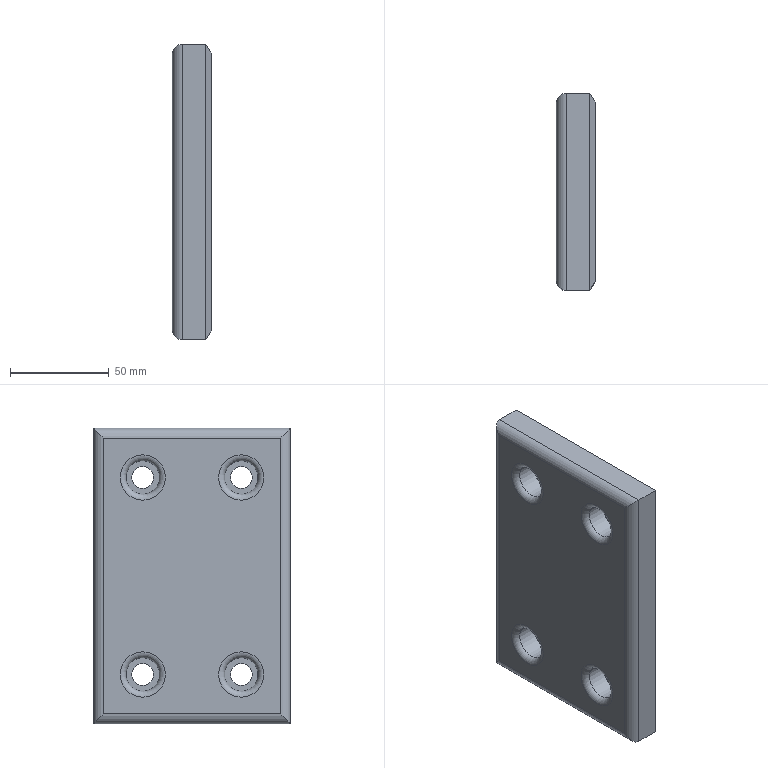Part | NX | features solid 2 | 1 solid | 30 faces | box 20 x 100 x 150 mm | volume 278806 mm3 | plane 14 | cylinder 12 | torus 4 | commonest cylinder face diameters 10 x4 11 x4 17 x4
STEP:
#1=CARTESIAN_POINT('',(-1412.,120.,-125.5));
#2=VERTEX_POINT('',#1);
#3=CARTESIAN_POINT('',(-1412.,120.,-120.));
#4=DIRECTION('',(1.,0.,0.));
#5=DIRECTION('',(0.,0.,-1.));
#6=AXIS2_PLACEMENT_3D('',#3,#4,#5);
#7=CIRCLE('',#6,5.5);
#8=EDGE_CURVE('',#2,#2,#7,.T.);
#9=ORIENTED_EDGE('',*,*,#8,.T.);
#10=EDGE_LOOP('',(#9));
#11=FACE_BOUND('',#10,.T.);
#12=CARTESIAN_POINT('',(-1412.,120.,-128.5));
#13=VERTEX_POINT('',#12);
#14=CARTESIAN_POINT('',(-1412.,120.,-120.));
#15=DIRECTION('',(1.,0.,0.));
#16=DIRECTION('',(0.,0.,-1.));
#17=AXIS2_PLACEMENT_3D('',#14,#15,#16);
#18=CIRCLE('',#17,8.5);
#19=EDGE_CURVE('',#13,#13,#18,.T.);
#20=ORIENTED_EDGE('',*,*,#19,.F.);
#21=EDGE_LOOP('',(#20));
#22=FACE_BOUND('',#21,.T.);
#23=CARTESIAN_POINT('',(-1412.,120.,-120.));
#24=DIRECTION('',(1.,0.,0.));
#25=DIRECTION('',(0.,0.,-1.));
#26=AXIS2_PLACEMENT_3D('',#23,#24,#25);
#27=PLANE('',#26);
#28=ADVANCED_FACE('',(#11,#22),#27,.F.);
#29=CARTESIAN_POINT('',(-1412.,70.,-125.5));
#30=VERTEX_POINT('',#29);
#31=CARTESIAN_POINT('',(-1412.,70.,-120.));
#32=DIRECTION('',(1.,0.,0.));
#33=DIRECTION('',(0.,0.,-1.));
#34=AXIS2_PLACEMENT_3D('',#31,#32,#33);
#35=CIRCLE('',#34,5.5);
#36=EDGE_CURVE('',#30,#30,#35,.T.);
#37=ORIENTED_EDGE('',*,*,#36,.T.);
#38=EDGE_LOOP('',(#37));
#39=FACE_BOUND('',#38,.T.);
#40=CARTESIAN_POINT('',(-1412.,70.,-128.5));
#41=VERTEX_POINT('',#40);
#42=CARTESIAN_POINT('',(-1412.,70.,-120.));
#43=DIRECTION('',(1.,0.,0.));
#44=DIRECTION('',(0.,0.,-1.));
#45=AXIS2_PLACEMENT_3D('',#42,#43,#44);
#46=CIRCLE('',#45,8.5);
#47=EDGE_CURVE('',#41,#41,#46,.T.);
#48=ORIENTED_EDGE('',*,*,#47,.F.);
#49=EDGE_LOOP('',(#48));
#50=FACE_BOUND('',#49,.T.);
#51=CARTESIAN_POINT('',(-1412.,70.,-120.));
#52=DIRECTION('',(1.,0.,0.));
#53=DIRECTION('',(0.,0.,-1.));
#54=AXIS2_PLACEMENT_3D('',#51,#52,#53);
#55=PLANE('',#54);
#56=ADVANCED_FACE('',(#39,#50),#55,.F.);
#57=CARTESIAN_POINT('',(-1422.,120.,-111.5));
#58=VERTEX_POINT('',#57);
#59=CARTESIAN_POINT('',(-1422.,120.,-120.));
#60=DIRECTION('',(-1.,0.,0.));
#61=DIRECTION('',(0.,0.,1.));
#62=AXIS2_PLACEMENT_3D('',#59,#60,#61);
#63=CIRCLE('',#62,8.5);
#64=EDGE_CURVE('',#58,#58,#63,.T.);
#65=ORIENTED_EDGE('',*,*,#64,.T.);
#66=EDGE_LOOP('',(#65));
#67=FACE_BOUND('',#66,.T.);
#68=ORIENTED_EDGE('',*,*,#19,.T.);
#69=EDGE_LOOP('',(#68));
#70=FACE_BOUND('',#69,.T.);
#71=CARTESIAN_POINT('',(-1425.,120.,-120.));
#72=DIRECTION('',(1.,0.,0.));
#73=DIRECTION('',(0.,0.,-1.));
#74=AXIS2_PLACEMENT_3D('',#71,#72,#73);
#75=CYLINDRICAL_SURFACE('',#74,8.5);
#76=ADVANCED_FACE('',(#67,#70),#75,.F.);
#77=CARTESIAN_POINT('',(-1422.,70.,-111.5));
#78=VERTEX_POINT('',#77);
#79=CARTESIAN_POINT('',(-1422.,70.,-120.));
#80=DIRECTION('',(-1.,0.,0.));
#81=DIRECTION('',(0.,0.,1.));
#82=AXIS2_PLACEMENT_3D('',#79,#80,#81);
#83=CIRCLE('',#82,8.5);
#84=EDGE_CURVE('',#78,#78,#83,.T.);
#85=ORIENTED_EDGE('',*,*,#84,.T.);
#86=EDGE_LOOP('',(#85));
#87=FACE_BOUND('',#86,.T.);
#88=ORIENTED_EDGE('',*,*,#47,.T.);
#89=EDGE_LOOP('',(#88));
#90=FACE_BOUND('',#89,.T.);
#91=CARTESIAN_POINT('',(-1425.,70.,-120.));
#92=DIRECTION('',(1.,0.,0.));
#93=DIRECTION('',(0.,0.,-1.));
#94=AXIS2_PLACEMENT_3D('',#91,#92,#93);
#95=CYLINDRICAL_SURFACE('',#94,8.5);
#96=ADVANCED_FACE('',(#87,#90),#95,.F.);
#97=ORIENTED_EDGE('',*,*,#8,.F.);
#98=EDGE_LOOP('',(#97));
#99=FACE_BOUND('',#98,.T.);
#100=CARTESIAN_POINT('',(-1405.,120.,-114.5));
#101=VERTEX_POINT('',#100);
#102=CARTESIAN_POINT('',(-1405.,120.,-120.));
#103=DIRECTION('',(-1.,0.,0.));
#104=DIRECTION('',(0.,0.,1.));
#105=AXIS2_PLACEMENT_3D('',#102,#103,#104);
#106=CIRCLE('',#105,5.5);
#107=EDGE_CURVE('',#101,#101,#106,.T.);
#108=ORIENTED_EDGE('',*,*,#107,.F.);
#109=EDGE_LOOP('',(#108));
#110=FACE_BOUND('',#109,.T.);
#111=CARTESIAN_POINT('',(-1375.,120.,-120.));
#112=DIRECTION('',(1.,0.,0.));
#113=DIRECTION('',(0.,0.,-1.));
#114=AXIS2_PLACEMENT_3D('',#111,#112,#113);
#115=CYLINDRICAL_SURFACE('',#114,5.5);
#116=ADVANCED_FACE('',(#99,#110),#115,.F.);
#117=ORIENTED_EDGE('',*,*,#36,.F.);
#118=EDGE_LOOP('',(#117));
#119=FACE_BOUND('',#118,.T.);
#120=CARTESIAN_POINT('',(-1405.,70.,-114.5));
#121=VERTEX_POINT('',#120);
#122=CARTESIAN_POINT('',(-1405.,70.,-120.));
#123=DIRECTION('',(-1.,0.,0.));
#124=DIRECTION('',(0.,0.,1.));
#125=AXIS2_PLACEMENT_3D('',#122,#123,#124);
#126=CIRCLE('',#125,5.5);
#127=EDGE_CURVE('',#121,#121,#126,.T.);
#128=ORIENTED_EDGE('',*,*,#127,.F.);
#129=EDGE_LOOP('',(#128));
#130=FACE_BOUND('',#129,.T.);
#131=CARTESIAN_POINT('',(-1375.,70.,-120.));
#132=DIRECTION('',(1.,0.,0.));
#133=DIRECTION('',(0.,0.,-1.));
#134=AXIS2_PLACEMENT_3D('',#131,#132,#133);
#135=CYLINDRICAL_SURFACE('',#134,5.5);
#136=ADVANCED_FACE('',(#119,#130),#135,.F.);
#137=CARTESIAN_POINT('',(-1420.,145.,-145.));
#138=VERTEX_POINT('',#137);
#139=CARTESIAN_POINT('',(-1408.,145.,-145.));
#140=VERTEX_POINT('',#139);
#141=CARTESIAN_POINT('',(-1425.,145.,-145.));
#142=DIRECTION('',(-1.,0.,0.));
#143=VECTOR('',#142,1000.);
#144=LINE('',#141,#143);
#145=EDGE_CURVE('',#138,#140,#144,.F.);
#146=ORIENTED_EDGE('',*,*,#145,.T.);
#147=CARTESIAN_POINT('',(-1408.,45.,-145.));
#148=VERTEX_POINT('',#147);
#149=CARTESIAN_POINT('',(-1408.,135.,-145.));
#150=DIRECTION('',(0.,1.,0.));
#151=VECTOR('',#150,1000.);
#152=LINE('',#149,#151);
#153=EDGE_CURVE('',#140,#148,#152,.F.);
#154=ORIENTED_EDGE('',*,*,#153,.T.);
#155=CARTESIAN_POINT('',(-1420.,45.,-145.));
#156=VERTEX_POINT('',#155);
#157=CARTESIAN_POINT('',(-1425.,45.,-145.));
#158=DIRECTION('',(-1.,0.,0.));
#159=VECTOR('',#158,1000.);
#160=LINE('',#157,#159);
#161=EDGE_CURVE('',#156,#148,#160,.F.);
#162=ORIENTED_EDGE('',*,*,#161,.F.);
#163=CARTESIAN_POINT('',(-1420.,145.,-145.));
#164=DIRECTION('',(0.,1.,0.));
#165=VECTOR('',#164,1000.);
#166=LINE('',#163,#165);
#167=EDGE_CURVE('',#156,#138,#166,.T.);
#168=ORIENTED_EDGE('',*,*,#167,.T.);
#169=EDGE_LOOP('',(#146,#154,#162,#168));
#170=FACE_BOUND('',#169,.T.);
#171=CARTESIAN_POINT('',(-1415.,135.,-145.));
#172=DIRECTION('',(0.,0.,-1.));
#173=DIRECTION('',(0.,-1.,0.));
#174=AXIS2_PLACEMENT_3D('',#171,#172,#173);
#175=PLANE('',#174);
#176=ADVANCED_FACE('',(#170),#175,.T.);
#177=ORIENTED_EDGE('',*,*,#64,.F.);
#178=EDGE_LOOP('',(#177));
#179=FACE_BOUND('',#178,.T.);
#180=CARTESIAN_POINT('',(-1425.,120.,-108.5));
#181=VERTEX_POINT('',#180);
#182=CARTESIAN_POINT('',(-1425.,120.,-120.));
#183=DIRECTION('',(-1.,0.,0.));
#184=DIRECTION('',(0.,0.,1.));
#185=AXIS2_PLACEMENT_3D('',#182,#183,#184);
#186=CIRCLE('',#185,11.5);
#187=EDGE_CURVE('',#181,#181,#186,.F.);
#188=ORIENTED_EDGE('',*,*,#187,.F.);
#189=EDGE_LOOP('',(#188));
#190=FACE_BOUND('',#189,.T.);
#191=CARTESIAN_POINT('',(-1422.,120.,-120.));
#192=DIRECTION('',(-1.,0.,0.));
#193=DIRECTION('',(0.,0.,1.));
#194=AXIS2_PLACEMENT_3D('',#191,#192,#193);
#195=TOROIDAL_SURFACE('',#194,11.5,3.);
#196=ADVANCED_FACE('',(#179,#190),#195,.T.);
#197=ORIENTED_EDGE('',*,*,#84,.F.);
#198=EDGE_LOOP('',(#197));
#199=FACE_BOUND('',#198,.T.);
#200=CARTESIAN_POINT('',(-1425.,70.,-108.5));
#201=VERTEX_POINT('',#200);
#202=CARTESIAN_POINT('',(-1425.,70.,-120.));
#203=DIRECTION('',(-1.,0.,0.));
#204=DIRECTION('',(0.,0.,1.));
#205=AXIS2_PLACEMENT_3D('',#202,#203,#204);
#206=CIRCLE('',#205,11.5);
#207=EDGE_CURVE('',#201,#201,#206,.F.);
#208=ORIENTED_EDGE('',*,*,#207,.F.);
#209=EDGE_LOOP('',(#208));
#210=FACE_BOUND('',#209,.T.);
#211=CARTESIAN_POINT('',(-1422.,70.,-120.));
#212=DIRECTION('',(-1.,0.,0.));
#213=DIRECTION('',(0.,0.,1.));
#214=AXIS2_PLACEMENT_3D('',#211,#212,#213);
#215=TOROIDAL_SURFACE('',#214,11.5,3.);
#216=ADVANCED_FACE('',(#199,#210),#215,.T.);
#217=CARTESIAN_POINT('',(-1425.,50.,-140.));
#218=VERTEX_POINT('',#217);
#219=CARTESIAN_POINT('',(-1420.,50.,-140.));
#220=DIRECTION('',(0.,-0.7071,0.7071));
#221=DIRECTION('',(0.,0.7071,0.7071));
#222=AXIS2_PLACEMENT_3D('',#219,#220,#221);
#223=ELLIPSE('',#222,7.071,5.);
#224=EDGE_CURVE('',#156,#218,#223,.F.);
#225=ORIENTED_EDGE('',*,*,#224,.T.);
#226=CARTESIAN_POINT('',(-1425.,140.,-140.));
#227=VERTEX_POINT('',#226);
#228=CARTESIAN_POINT('',(-1425.,45.,-140.));
#229=DIRECTION('',(0.,-1.,0.));
#230=VECTOR('',#229,1000.);
#231=LINE('',#228,#230);
#232=EDGE_CURVE('',#227,#218,#231,.T.);
#233=ORIENTED_EDGE('',*,*,#232,.F.);
#234=CARTESIAN_POINT('',(-1420.,140.,-140.));
#235=DIRECTION('',(0.,-0.7071,-0.7071));
#236=DIRECTION('',(0.,0.7071,-0.7071));
#237=AXIS2_PLACEMENT_3D('',#234,#235,#236);
#238=ELLIPSE('',#237,7.071,5.);
#239=EDGE_CURVE('',#227,#138,#238,.T.);
#240=ORIENTED_EDGE('',*,*,#239,.T.);
#241=ORIENTED_EDGE('',*,*,#167,.F.);
#242=EDGE_LOOP('',(#225,#233,#240,#241));
#243=FACE_BOUND('',#242,.T.);
#244=CARTESIAN_POINT('',(-1420.,135.,-140.));
#245=DIRECTION('',(0.,1.,0.));
#246=DIRECTION('',(0.,0.,1.));
#247=AXIS2_PLACEMENT_3D('',#244,#245,#246);
#248=CYLINDRICAL_SURFACE('',#247,5.);
#249=ADVANCED_FACE('',(#243),#248,.T.);
#250=CARTESIAN_POINT('',(-1405.,50.,-140.));
#251=VERTEX_POINT('',#250);
#252=CARTESIAN_POINT('',(-1248.644,310.593,120.593));
#253=DIRECTION('',(-0.3906,-0.6509,-0.6509));
#254=VECTOR('',#253,1000.);
#255=LINE('',#252,#254);
#256=EDGE_CURVE('',#251,#148,#255,.T.);
#257=ORIENTED_EDGE('',*,*,#256,.T.);
#258=ORIENTED_EDGE('',*,*,#153,.F.);
#259=CARTESIAN_POINT('',(-1405.,140.,-140.));
#260=VERTEX_POINT('',#259);
#261=CARTESIAN_POINT('',(-1250.373,-117.712,117.712));
#262=DIRECTION('',(-0.3906,0.6509,-0.6509));
#263=VECTOR('',#262,1000.);
#264=LINE('',#261,#263);
#265=EDGE_CURVE('',#140,#260,#264,.F.);
#266=ORIENTED_EDGE('',*,*,#265,.T.);
#267=CARTESIAN_POINT('',(-1405.,45.,-140.));
#268=DIRECTION('',(0.,1.,0.));
#269=VECTOR('',#268,1000.);
#270=LINE('',#267,#269);
#271=EDGE_CURVE('',#251,#260,#270,.T.);
#272=ORIENTED_EDGE('',*,*,#271,.F.);
#273=EDGE_LOOP('',(#257,#258,#266,#272));
#274=FACE_BOUND('',#273,.T.);
#275=CARTESIAN_POINT('',(-1405.,45.,-140.));
#276=DIRECTION('',(0.8575,0.,-0.5145));
#277=DIRECTION('',(-0.5145,0.,-0.8575));
#278=AXIS2_PLACEMENT_3D('',#275,#276,#277);
#279=PLANE('',#278);
#280=ADVANCED_FACE('',(#274),#279,.T.);
#281=CARTESIAN_POINT('',(-1420.,45.,5.));
#282=VERTEX_POINT('',#281);
#283=CARTESIAN_POINT('',(-1420.,45.,-145.));
#284=DIRECTION('',(0.,0.,-1.));
#285=VECTOR('',#284,1000.);
#286=LINE('',#283,#285);
#287=EDGE_CURVE('',#282,#156,#286,.T.);
#288=ORIENTED_EDGE('',*,*,#287,.F.);
#289=CARTESIAN_POINT('',(-1425.,50.,0.));
#290=VERTEX_POINT('',#289);
#291=CARTESIAN_POINT('',(-1420.,50.,0.));
#292=DIRECTION('',(0.,0.7071,0.7071));
#293=DIRECTION('',(0.,0.7071,-0.7071));
#294=AXIS2_PLACEMENT_3D('',#291,#292,#293);
#295=ELLIPSE('',#294,7.071,5.);
#296=EDGE_CURVE('',#282,#290,#295,.F.);
#297=ORIENTED_EDGE('',*,*,#296,.T.);
#298=CARTESIAN_POINT('',(-1425.,50.,-20.));
#299=DIRECTION('',(0.,0.,-1.));
#300=VECTOR('',#299,1000.);
#301=LINE('',#298,#300);
#302=EDGE_CURVE('',#218,#290,#301,.F.);
#303=ORIENTED_EDGE('',*,*,#302,.F.);
#304=ORIENTED_EDGE('',*,*,#224,.F.);
#305=EDGE_LOOP('',(#288,#297,#303,#304));
#306=FACE_BOUND('',#305,.T.);
#307=CARTESIAN_POINT('',(-1420.,50.,475.));
#308=DIRECTION('',(0.,0.,1.));
#309=DIRECTION('',(1.,0.,0.));
#310=AXIS2_PLACEMENT_3D('',#307,#308,#309);
#311=CYLINDRICAL_SURFACE('',#310,5.);
#312=ADVANCED_FACE('',(#306),#311,.T.);
#313=CARTESIAN_POINT('',(-1425.,140.,0.));
#314=VERTEX_POINT('',#313);
#315=CARTESIAN_POINT('',(-1425.,140.,475.));
#316=DIRECTION('',(0.,0.,-1.));
#317=VECTOR('',#316,1000.);
#318=LINE('',#315,#317);
#319=EDGE_CURVE('',#314,#227,#318,.T.);
#320=ORIENTED_EDGE('',*,*,#319,.F.);
#321=CARTESIAN_POINT('',(-1420.,145.,5.));
#322=VERTEX_POINT('',#321);
#323=CARTESIAN_POINT('',(-1420.,140.,0.));
#324=DIRECTION('',(0.,0.7071,-0.7071));
#325=DIRECTION('',(0.,0.7071,0.7071));
#326=AXIS2_PLACEMENT_3D('',#323,#324,#325);
#327=ELLIPSE('',#326,7.071,5.);
#328=EDGE_CURVE('',#314,#322,#327,.T.);
#329=ORIENTED_EDGE('',*,*,#328,.T.);
#330=CARTESIAN_POINT('',(-1420.,145.,475.));
#331=DIRECTION('',(0.,0.,-1.));
#332=VECTOR('',#331,1000.);
#333=LINE('',#330,#332);
#334=EDGE_CURVE('',#138,#322,#333,.F.);
#335=ORIENTED_EDGE('',*,*,#334,.F.);
#336=ORIENTED_EDGE('',*,*,#239,.F.);
#337=EDGE_LOOP('',(#320,#329,#335,#336));
#338=FACE_BOUND('',#337,.T.);
#339=CARTESIAN_POINT('',(-1420.,140.,475.));
#340=DIRECTION('',(0.,0.,-1.));
#341=DIRECTION('',(-1.,0.,0.));
#342=AXIS2_PLACEMENT_3D('',#339,#340,#341);
#343=CYLINDRICAL_SURFACE('',#342,5.);
#344=ADVANCED_FACE('',(#338),#343,.T.);
#345=ORIENTED_EDGE('',*,*,#302,.T.);
#346=CARTESIAN_POINT('',(-1425.,45.,0.));
#347=DIRECTION('',(0.,1.,0.));
#348=VECTOR('',#347,1000.);
#349=LINE('',#346,#348);
#350=EDGE_CURVE('',#290,#314,#349,.T.);
#351=ORIENTED_EDGE('',*,*,#350,.T.);
#352=ORIENTED_EDGE('',*,*,#319,.T.);
#353=ORIENTED_EDGE('',*,*,#232,.T.);
#354=EDGE_LOOP('',(#345,#351,#352,#353));
#355=FACE_BOUND('',#354,.T.);
#356=ORIENTED_EDGE('',*,*,#207,.T.);
#357=EDGE_LOOP('',(#356));
#358=FACE_BOUND('',#357,.T.);
#359=ORIENTED_EDGE('',*,*,#187,.T.);
#360=EDGE_LOOP('',(#359));
#361=FACE_BOUND('',#360,.T.);
#362=CARTESIAN_POINT('',(-1425.,120.,-8.5));
#363=VERTEX_POINT('',#362);
#364=CARTESIAN_POINT('',(-1425.,120.,-20.));
#365=DIRECTION('',(-1.,0.,0.));
#366=DIRECTION('',(0.,0.,1.));
#367=AXIS2_PLACEMENT_3D('',#364,#365,#366);
#368=CIRCLE('',#367,11.5);
#369=EDGE_CURVE('',#363,#363,#368,.F.);
#370=ORIENTED_EDGE('',*,*,#369,.T.);
#371=EDGE_LOOP('',(#370));
#372=FACE_BOUND('',#371,.T.);
#373=CARTESIAN_POINT('',(-1425.,70.,-8.5));
#374=VERTEX_POINT('',#373);
#375=CARTESIAN_POINT('',(-1425.,70.,-20.));
#376=DIRECTION('',(-1.,0.,0.));
#377=DIRECTION('',(0.,0.,1.));
#378=AXIS2_PLACEMENT_3D('',#375,#376,#377);
#379=CIRCLE('',#378,11.5);
#380=EDGE_CURVE('',#374,#374,#379,.F.);
#381=ORIENTED_EDGE('',*,*,#380,.T.);
#382=EDGE_LOOP('',(#381));
#383=FACE_BOUND('',#382,.T.);
#384=CARTESIAN_POINT('',(-1425.,45.,475.));
#385=DIRECTION('',(-1.,0.,0.));
#386=DIRECTION('',(0.,0.,1.));
#387=AXIS2_PLACEMENT_3D('',#384,#385,#386);
#388=PLANE('',#387);
#389=ADVANCED_FACE('',(#355,#358,#361,#372,#383),#388,.T.);
#390=CARTESIAN_POINT('',(-1405.,50.,0.));
#391=VERTEX_POINT('',#390);
#392=CARTESIAN_POINT('',(-1405.,50.,475.));
#393=DIRECTION('',(0.,0.,-1.));
#394=VECTOR('',#393,1000.);
#395=LINE('',#392,#394);
#396=EDGE_CURVE('',#391,#251,#395,.T.);
#397=ORIENTED_EDGE('',*,*,#396,.F.);
#398=CARTESIAN_POINT('',(-1408.,45.,5.));
#399=VERTEX_POINT('',#398);
#400=CARTESIAN_POINT('',(-1425.797,15.339,34.661));
#401=DIRECTION('',(-0.3906,-0.6509,0.6509));
#402=VECTOR('',#401,1000.);
#403=LINE('',#400,#402);
#404=EDGE_CURVE('',#391,#399,#403,.T.);
#405=ORIENTED_EDGE('',*,*,#404,.T.);
#406=CARTESIAN_POINT('',(-1408.,45.,475.));
#407=DIRECTION('',(0.,0.,1.));
#408=VECTOR('',#407,1000.);
#409=LINE('',#406,#408);
#410=EDGE_CURVE('',#148,#399,#409,.T.);
#411=ORIENTED_EDGE('',*,*,#410,.F.);
#412=ORIENTED_EDGE('',*,*,#256,.F.);
#413=EDGE_LOOP('',(#397,#405,#411,#412));
#414=FACE_BOUND('',#413,.T.);
#415=CARTESIAN_POINT('',(-1405.,50.,475.));
#416=DIRECTION('',(-0.8575,0.5145,0.));
#417=DIRECTION('',(-0.5145,-0.8575,0.));
#418=AXIS2_PLACEMENT_3D('',#415,#416,#417);
#419=PLANE('',#418);
#420=ADVANCED_FACE('',(#414),#419,.F.);
#421=ORIENTED_EDGE('',*,*,#410,.T.);
#422=CARTESIAN_POINT('',(-1425.,45.,5.));
#423=DIRECTION('',(1.,0.,0.));
#424=VECTOR('',#423,1000.);
#425=LINE('',#422,#424);
#426=EDGE_CURVE('',#282,#399,#425,.T.);
#427=ORIENTED_EDGE('',*,*,#426,.F.);
#428=ORIENTED_EDGE('',*,*,#287,.T.);
#429=ORIENTED_EDGE('',*,*,#161,.T.);
#430=EDGE_LOOP('',(#421,#427,#428,#429));
#431=FACE_BOUND('',#430,.T.);
#432=CARTESIAN_POINT('',(-1425.,45.,475.));
#433=DIRECTION('',(0.,1.,0.));
#434=DIRECTION('',(0.,0.,1.));
#435=AXIS2_PLACEMENT_3D('',#432,#433,#434);
#436=PLANE('',#435);
#437=ADVANCED_FACE('',(#431),#436,.F.);
#438=CARTESIAN_POINT('',(-1408.,145.,5.));
#439=VERTEX_POINT('',#438);
#440=CARTESIAN_POINT('',(-1408.,145.,-145.));
#441=DIRECTION('',(0.,0.,-1.));
#442=VECTOR('',#441,1000.);
#443=LINE('',#440,#442);
#444=EDGE_CURVE('',#439,#140,#443,.T.);
#445=ORIENTED_EDGE('',*,*,#444,.F.);
#446=CARTESIAN_POINT('',(-1405.,140.,0.));
#447=VERTEX_POINT('',#446);
#448=CARTESIAN_POINT('',(-1533.847,354.746,214.746));
#449=DIRECTION('',(0.3906,-0.6509,-0.6509));
#450=VECTOR('',#449,1000.);
#451=LINE('',#448,#450);
#452=EDGE_CURVE('',#439,#447,#451,.T.);
#453=ORIENTED_EDGE('',*,*,#452,.T.);
#454=CARTESIAN_POINT('',(-1405.,140.,-20.));
#455=DIRECTION('',(0.,0.,1.));
#456=VECTOR('',#455,1000.);
#457=LINE('',#454,#456);
#458=EDGE_CURVE('',#260,#447,#457,.T.);
#459=ORIENTED_EDGE('',*,*,#458,.F.);
#460=ORIENTED_EDGE('',*,*,#265,.F.);
#461=EDGE_LOOP('',(#445,#453,#459,#460));
#462=FACE_BOUND('',#461,.T.);
#463=CARTESIAN_POINT('',(-1408.,145.,475.));
#464=DIRECTION('',(0.8575,0.5145,0.));
#465=DIRECTION('',(-0.5145,0.8575,0.));
#466=AXIS2_PLACEMENT_3D('',#463,#464,#465);
#467=PLANE('',#466);
#468=ADVANCED_FACE('',(#462),#467,.T.);
#469=ORIENTED_EDGE('',*,*,#458,.T.);
#470=CARTESIAN_POINT('',(-1405.,45.,0.));
#471=DIRECTION('',(0.,-1.,0.));
#472=VECTOR('',#471,1000.);
#473=LINE('',#470,#472);
#474=EDGE_CURVE('',#447,#391,#473,.T.);
#475=ORIENTED_EDGE('',*,*,#474,.T.);
#476=ORIENTED_EDGE('',*,*,#396,.T.);
#477=ORIENTED_EDGE('',*,*,#271,.T.);
#478=EDGE_LOOP('',(#469,#475,#476,#477));
#479=FACE_BOUND('',#478,.T.);
#480=ORIENTED_EDGE('',*,*,#127,.T.);
#481=EDGE_LOOP('',(#480));
#482=FACE_BOUND('',#481,.T.);
#483=ORIENTED_EDGE('',*,*,#107,.T.);
#484=EDGE_LOOP('',(#483));
#485=FACE_BOUND('',#484,.T.);
#486=CARTESIAN_POINT('',(-1405.,120.,-14.5));
#487=VERTEX_POINT('',#486);
#488=CARTESIAN_POINT('',(-1405.,120.,-20.));
#489=DIRECTION('',(-1.,0.,0.));
#490=DIRECTION('',(0.,0.,1.));
#491=AXIS2_PLACEMENT_3D('',#488,#489,#490);
#492=CIRCLE('',#491,5.5);
#493=EDGE_CURVE('',#487,#487,#492,.T.);
#494=ORIENTED_EDGE('',*,*,#493,.T.);
#495=EDGE_LOOP('',(#494));
#496=FACE_BOUND('',#495,.T.);
#497=CARTESIAN_POINT('',(-1405.,70.,-14.5));
#498=VERTEX_POINT('',#497);
#499=CARTESIAN_POINT('',(-1405.,70.,-20.));
#500=DIRECTION('',(-1.,0.,0.));
#501=DIRECTION('',(0.,0.,1.));
#502=AXIS2_PLACEMENT_3D('',#499,#500,#501);
#503=CIRCLE('',#502,5.5);
#504=EDGE_CURVE('',#498,#498,#503,.T.);
#505=ORIENTED_EDGE('',*,*,#504,.T.);
#506=EDGE_LOOP('',(#505));
#507=FACE_BOUND('',#506,.T.);
#508=CARTESIAN_POINT('',(-1405.,45.,475.));
#509=DIRECTION('',(-1.,0.,0.));
#510=DIRECTION('',(0.,0.,1.));
#511=AXIS2_PLACEMENT_3D('',#508,#509,#510);
#512=PLANE('',#511);
#513=ADVANCED_FACE('',(#479,#482,#485,#496,#507),#512,.F.);
#514=ORIENTED_EDGE('',*,*,#334,.T.);
#515=CARTESIAN_POINT('',(-1425.,145.,5.));
#516=DIRECTION('',(1.,0.,0.));
#517=VECTOR('',#516,1000.);
#518=LINE('',#515,#517);
#519=EDGE_CURVE('',#322,#439,#518,.T.);
#520=ORIENTED_EDGE('',*,*,#519,.T.);
#521=ORIENTED_EDGE('',*,*,#444,.T.);
#522=ORIENTED_EDGE('',*,*,#145,.F.);
#523=EDGE_LOOP('',(#514,#520,#521,#522));
#524=FACE_BOUND('',#523,.T.);
#525=CARTESIAN_POINT('',(-1425.,145.,475.));
#526=DIRECTION('',(0.,1.,0.));
#527=DIRECTION('',(0.,0.,1.));
#528=AXIS2_PLACEMENT_3D('',#525,#526,#527);
#529=PLANE('',#528);
#530=ADVANCED_FACE('',(#524),#529,.T.);
#531=ORIENTED_EDGE('',*,*,#426,.T.);
#532=CARTESIAN_POINT('',(-1408.,145.,5.));
#533=DIRECTION('',(0.,1.,0.));
#534=VECTOR('',#533,1000.);
#535=LINE('',#532,#534);
#536=EDGE_CURVE('',#399,#439,#535,.T.);
#537=ORIENTED_EDGE('',*,*,#536,.T.);
#538=ORIENTED_EDGE('',*,*,#519,.F.);
#539=CARTESIAN_POINT('',(-1420.,-25.,5.));
#540=DIRECTION('',(0.,1.,0.));
#541=VECTOR('',#540,1000.);
#542=LINE('',#539,#541);
#543=EDGE_CURVE('',#322,#282,#542,.F.);
#544=ORIENTED_EDGE('',*,*,#543,.T.);
#545=EDGE_LOOP('',(#531,#537,#538,#544));
#546=FACE_BOUND('',#545,.T.);
#547=CARTESIAN_POINT('',(-1470.,-25.,5.));
#548=DIRECTION('',(0.,0.,1.));
#549=DIRECTION('',(1.,0.,0.));
#550=AXIS2_PLACEMENT_3D('',#547,#548,#549);
#551=PLANE('',#550);
#552=ADVANCED_FACE('',(#546),#551,.T.);
#553=CARTESIAN_POINT('',(-1412.,120.,-25.5));
#554=VERTEX_POINT('',#553);
#555=CARTESIAN_POINT('',(-1412.,120.,-20.));
#556=DIRECTION('',(1.,0.,0.));
#557=DIRECTION('',(0.,0.,-1.));
#558=AXIS2_PLACEMENT_3D('',#555,#556,#557);
#559=CIRCLE('',#558,5.5);
#560=EDGE_CURVE('',#554,#554,#559,.T.);
#561=ORIENTED_EDGE('',*,*,#560,.F.);
#562=EDGE_LOOP('',(#561));
#563=FACE_BOUND('',#562,.T.);
#564=ORIENTED_EDGE('',*,*,#493,.F.);
#565=EDGE_LOOP('',(#564));
#566=FACE_BOUND('',#565,.T.);
#567=CARTESIAN_POINT('',(-1375.,120.,-20.));
#568=DIRECTION('',(1.,0.,0.));
#569=DIRECTION('',(0.,0.,-1.));
#570=AXIS2_PLACEMENT_3D('',#567,#568,#569);
#571=CYLINDRICAL_SURFACE('',#570,5.5);
#572=ADVANCED_FACE('',(#563,#566),#571,.F.);
#573=ORIENTED_EDGE('',*,*,#560,.T.);
#574=EDGE_LOOP('',(#573));
#575=FACE_BOUND('',#574,.T.);
#576=CARTESIAN_POINT('',(-1412.,120.,-28.5));
#577=VERTEX_POINT('',#576);
#578=CARTESIAN_POINT('',(-1412.,120.,-20.));
#579=DIRECTION('',(1.,0.,0.));
#580=DIRECTION('',(0.,0.,-1.));
#581=AXIS2_PLACEMENT_3D('',#578,#579,#580);
#582=CIRCLE('',#581,8.5);
#583=EDGE_CURVE('',#577,#577,#582,.T.);
#584=ORIENTED_EDGE('',*,*,#583,.F.);
#585=EDGE_LOOP('',(#584));
#586=FACE_BOUND('',#585,.T.);
#587=CARTESIAN_POINT('',(-1412.,120.,-20.));
#588=DIRECTION('',(1.,0.,0.));
#589=DIRECTION('',(0.,0.,-1.));
#590=AXIS2_PLACEMENT_3D('',#587,#588,#589);
#591=PLANE('',#590);
#592=ADVANCED_FACE('',(#575,#586),#591,.F.);
#593=CARTESIAN_POINT('',(-1422.,120.,-11.5));
#594=VERTEX_POINT('',#593);
#595=CARTESIAN_POINT('',(-1422.,120.,-20.));
#596=DIRECTION('',(-1.,0.,0.));
#597=DIRECTION('',(0.,0.,1.));
#598=AXIS2_PLACEMENT_3D('',#595,#596,#597);
#599=CIRCLE('',#598,8.5);
#600=EDGE_CURVE('',#594,#594,#599,.T.);
#601=ORIENTED_EDGE('',*,*,#600,.T.);
#602=EDGE_LOOP('',(#601));
#603=FACE_BOUND('',#602,.T.);
#604=ORIENTED_EDGE('',*,*,#583,.T.);
#605=EDGE_LOOP('',(#604));
#606=FACE_BOUND('',#605,.T.);
#607=CARTESIAN_POINT('',(-1425.,120.,-20.));
#608=DIRECTION('',(1.,0.,0.));
#609=DIRECTION('',(0.,0.,-1.));
#610=AXIS2_PLACEMENT_3D('',#607,#608,#609);
#611=CYLINDRICAL_SURFACE('',#610,8.5);
#612=ADVANCED_FACE('',(#603,#606),#611,.F.);
#613=CARTESIAN_POINT('',(-1412.,70.,-25.5));
#614=VERTEX_POINT('',#613);
#615=CARTESIAN_POINT('',(-1412.,70.,-20.));
#616=DIRECTION('',(1.,0.,0.));
#617=DIRECTION('',(0.,0.,-1.));
#618=AXIS2_PLACEMENT_3D('',#615,#616,#617);
#619=CIRCLE('',#618,5.5);
#620=EDGE_CURVE('',#614,#614,#619,.T.);
#621=ORIENTED_EDGE('',*,*,#620,.F.);
#622=EDGE_LOOP('',(#621));
#623=FACE_BOUND('',#622,.T.);
#624=ORIENTED_EDGE('',*,*,#504,.F.);
#625=EDGE_LOOP('',(#624));
#626=FACE_BOUND('',#625,.T.);
#627=CARTESIAN_POINT('',(-1375.,70.,-20.));
#628=DIRECTION('',(1.,0.,0.));
#629=DIRECTION('',(0.,0.,-1.));
#630=AXIS2_PLACEMENT_3D('',#627,#628,#629);
#631=CYLINDRICAL_SURFACE('',#630,5.5);
#632=ADVANCED_FACE('',(#623,#626),#631,.F.);
#633=ORIENTED_EDGE('',*,*,#620,.T.);
#634=EDGE_LOOP('',(#633));
#635=FACE_BOUND('',#634,.T.);
#636=CARTESIAN_POINT('',(-1412.,70.,-28.5));
#637=VERTEX_POINT('',#636);
#638=CARTESIAN_POINT('',(-1412.,70.,-20.));
#639=DIRECTION('',(1.,0.,0.));
#640=DIRECTION('',(0.,0.,-1.));
#641=AXIS2_PLACEMENT_3D('',#638,#639,#640);
#642=CIRCLE('',#641,8.5);
#643=EDGE_CURVE('',#637,#637,#642,.T.);
#644=ORIENTED_EDGE('',*,*,#643,.F.);
#645=EDGE_LOOP('',(#644));
#646=FACE_BOUND('',#645,.T.);
#647=CARTESIAN_POINT('',(-1412.,70.,-20.));
#648=DIRECTION('',(1.,0.,0.));
#649=DIRECTION('',(0.,0.,-1.));
#650=AXIS2_PLACEMENT_3D('',#647,#648,#649);
#651=PLANE('',#650);
#652=ADVANCED_FACE('',(#635,#646),#651,.F.);
#653=CARTESIAN_POINT('',(-1422.,70.,-11.5));
#654=VERTEX_POINT('',#653);
#655=CARTESIAN_POINT('',(-1422.,70.,-20.));
#656=DIRECTION('',(-1.,0.,0.));
#657=DIRECTION('',(0.,0.,1.));
#658=AXIS2_PLACEMENT_3D('',#655,#656,#657);
#659=CIRCLE('',#658,8.5);
#660=EDGE_CURVE('',#654,#654,#659,.T.);
#661=ORIENTED_EDGE('',*,*,#660,.T.);
#662=EDGE_LOOP('',(#661));
#663=FACE_BOUND('',#662,.T.);
#664=ORIENTED_EDGE('',*,*,#643,.T.);
#665=EDGE_LOOP('',(#664));
#666=FACE_BOUND('',#665,.T.);
#667=CARTESIAN_POINT('',(-1425.,70.,-20.));
#668=DIRECTION('',(1.,0.,0.));
#669=DIRECTION('',(0.,0.,-1.));
#670=AXIS2_PLACEMENT_3D('',#667,#668,#669);
#671=CYLINDRICAL_SURFACE('',#670,8.5);
#672=ADVANCED_FACE('',(#663,#666),#671,.F.);
#673=ORIENTED_EDGE('',*,*,#660,.F.);
#674=EDGE_LOOP('',(#673));
#675=FACE_BOUND('',#674,.T.);
#676=ORIENTED_EDGE('',*,*,#380,.F.);
#677=EDGE_LOOP('',(#676));
#678=FACE_BOUND('',#677,.T.);
#679=CARTESIAN_POINT('',(-1422.,70.,-20.));
#680=DIRECTION('',(-1.,0.,0.));
#681=DIRECTION('',(0.,0.,1.));
#682=AXIS2_PLACEMENT_3D('',#679,#680,#681);
#683=TOROIDAL_SURFACE('',#682,11.5,3.);
#684=ADVANCED_FACE('',(#675,#678),#683,.T.);
#685=ORIENTED_EDGE('',*,*,#600,.F.);
#686=EDGE_LOOP('',(#685));
#687=FACE_BOUND('',#686,.T.);
#688=ORIENTED_EDGE('',*,*,#369,.F.);
#689=EDGE_LOOP('',(#688));
#690=FACE_BOUND('',#689,.T.);
#691=CARTESIAN_POINT('',(-1422.,120.,-20.));
#692=DIRECTION('',(-1.,0.,0.));
#693=DIRECTION('',(0.,0.,1.));
#694=AXIS2_PLACEMENT_3D('',#691,#692,#693);
#695=TOROIDAL_SURFACE('',#694,11.5,3.);
#696=ADVANCED_FACE('',(#687,#690),#695,.T.);
#697=ORIENTED_EDGE('',*,*,#328,.F.);
#698=ORIENTED_EDGE('',*,*,#350,.F.);
#699=ORIENTED_EDGE('',*,*,#296,.F.);
#700=ORIENTED_EDGE('',*,*,#543,.F.);
#701=EDGE_LOOP('',(#697,#698,#699,#700));
#702=FACE_BOUND('',#701,.T.);
#703=CARTESIAN_POINT('',(-1420.,45.,0.));
#704=DIRECTION('',(0.,1.,0.));
#705=DIRECTION('',(0.,0.,1.));
#706=AXIS2_PLACEMENT_3D('',#703,#704,#705);
#707=CYLINDRICAL_SURFACE('',#706,5.);
#708=ADVANCED_FACE('',(#702),#707,.T.);
#709=ORIENTED_EDGE('',*,*,#452,.F.);
#710=ORIENTED_EDGE('',*,*,#536,.F.);
#711=ORIENTED_EDGE('',*,*,#404,.F.);
#712=ORIENTED_EDGE('',*,*,#474,.F.);
#713=EDGE_LOOP('',(#709,#710,#711,#712));
#714=FACE_BOUND('',#713,.T.);
#715=CARTESIAN_POINT('',(-1408.,-25.,5.));
#716=DIRECTION('',(0.8575,0.,0.5145));
#717=DIRECTION('',(0.5145,0.,-0.8575));
#718=AXIS2_PLACEMENT_3D('',#715,#716,#717);
#719=PLANE('',#718);
#720=ADVANCED_FACE('',(#714),#719,.T.);
#721=CLOSED_SHELL('',(#28,#56,#76,#96,#116,#136,#176,#196,#216,#249,#280,#312,#344,#389,#420,#437,#468,#513,#530,#552,#572,#592,#612,#632,#652,#672,#684,#696,#708,#720));
#722=MANIFOLD_SOLID_BREP('',#721);
#723=(LENGTH_UNIT()NAMED_UNIT(*)SI_UNIT(.MILLI.,.METRE.));
#724=UNCERTAINTY_MEASURE_WITH_UNIT(LENGTH_MEASURE(0.00001),#723,'','');
#725=(NAMED_UNIT(*)PLANE_ANGLE_UNIT()SI_UNIT($,.RADIAN.));
#726=(NAMED_UNIT(*)SI_UNIT($,.STERADIAN.)SOLID_ANGLE_UNIT());
#727=(GEOMETRIC_REPRESENTATION_CONTEXT(3)GLOBAL_UNCERTAINTY_ASSIGNED_CONTEXT((#724))GLOBAL_UNIT_ASSIGNED_CONTEXT((#723,#725,#726))REPRESENTATION_CONTEXT('',''));
#728=ADVANCED_BREP_SHAPE_REPRESENTATION('',(#722),#727);